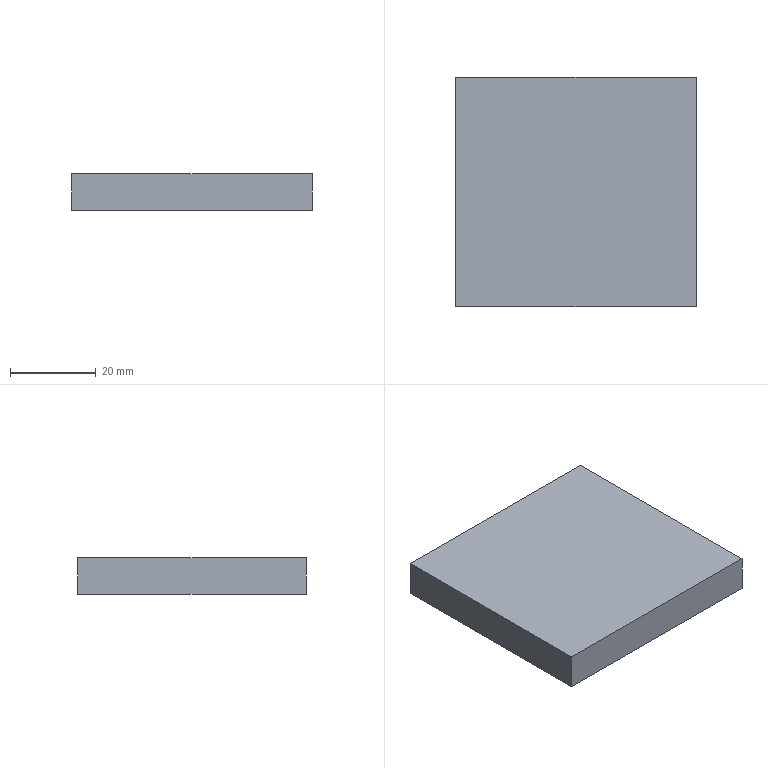NC program | NX | posted with a generic post | part box 56 x 53.3 x 8.5 mm
Lines 1 to 589 of 2943:
N10 G17 G21 G94 G90
(CAVITY_MILL_COPY_1 , TOOL : D6)
N12 T12 M6
N14 G54
N16 G17 G0 G90 X3.464 Y-2.284 S9500 M3
N18 G43 Z30. H12
N20 Z1.
N22 G94 G1 X3.837 Y-1.928 Z0.973 F800.
N24 X5.899 Y-0.453 Z0.84
N26 X6.766 Y0. Z0.789
N28 X5.899 Y0.453 Z0.738
N30 X3.837 Y1.928 Z0.605
N32 X2.861 Y2.861 Z0.534
N34 X1.928 Y3.837 Z0.463
N36 X0.453 Y5.899 Z0.33
N38 X0. Y6.766 Z0.279
N40 X-0.453 Y5.899 Z0.228
N42 X-1.928 Y3.837 Z0.095
N44 X-2.861 Y2.861 Z0.024
N46 X-3.837 Y1.928 Z-0.047
N48 X-5.899 Y0.453 Z-0.18
N50 X-6.766 Y0. Z-0.231
N52 X-5.899 Y-0.453 Z-0.282
N54 X-3.837 Y-1.928 Z-0.415
N56 X-2.995 Y-2.732 Z-0.476
N58 X-2.864 Y-2.864 Z-0.486
N60 X-0.318 Y-0.318
N62 G2 X0. Y-0.644 R19.55 F2500.
N64 X0.644 Y0. R19.55
N66 X0. Y0.644 R19.55
N68 X-0.644 Y0. R19.55
N70 X-0.318 Y-0.318 R19.55
N72 G1 X-2.864 Y-2.864
N74 G2 X0. Y-6.766 R15.95
N76 X6.766 Y0. R15.95
N78 X0. Y6.766 R15.95
N80 X-6.766 Y0. R15.95
N82 X-2.864 Y-2.864 R15.95
N84 G1 X-5.409 Y-5.409
N86 G2 X-2.162 Y-11.142 R12.35
N88 G3 X2.162 Y-11.142 R11.35
N90 G2 X11.73 Y-2.03 R12.35
N92 X12.671 Y-0.857 R11.3
N94 G3 X12.671 Y0.857 R12.7
N96 G2 X11.73 Y2.03 R11.3
N98 X2.162 Y11.142 R12.35
N100 G3 X-2.162 Y11.142 R11.35
N102 G2 X-11.73 Y2.03 R12.35
N104 X-12.671 Y0.857 R11.3
N106 G3 X-12.671 Y-0.857 R12.7
N108 G2 X-11.73 Y-2.03 R11.3
N110 X-5.409 Y-5.409 R12.35
N112 G1 X-7.955 Y-7.955
N114 G2 X-5.394 Y-13.943 R8.75
N116 G3 X5.394 Y-13.943 R14.95
N118 G2 X13.949 Y-5.394 R8.75
N120 X16.098 Y-2.557 R7.7
N122 G3 X16.098 Y2.557 R16.3
N124 G2 X13.949 Y5.394 R7.7
N126 X5.394 Y13.943 R8.75
N128 G3 X-5.394 Y13.943 R14.95
N130 G2 X-13.949 Y5.394 R8.75
N132 X-16.098 Y2.557 R7.7
N134 G3 X-16.098 Y-2.557 R16.3
N136 G2 X-13.949 Y-5.394 R7.7
N138 X-7.955 Y-7.955 R8.75
N140 G1 X-10.501 Y-10.501
N142 G2 X-9.348 Y-16.023 R5.15
N144 G3 X9.348 Y-16.022 R18.55
N146 G2 X16.023 Y-9.348 R5.15
N148 G3 X17.194 Y-6.961 R18.55
N150 G2 X19.323 Y-4.756 R4.1
N152 G3 X19.323 Y4.756 R19.9
N154 G2 X17.194 Y6.961 R4.1
N156 G3 X16.022 Y9.348 R18.55
N158 G2 X9.348 Y16.023 R5.15
N160 G3 X-9.348 Y16.023 R18.55
N162 G2 X-16.023 Y9.348 R5.15
N164 G3 X-17.194 Y6.961 R18.55
N166 G2 X-19.297 Y4.768 R4.1
N168 G1 X-19.325 Y4.75
N170 G3 X-19.325 Y-4.75 R19.9
N172 G1 X-19.297 Y-4.768
N174 G2 X-17.194 Y-6.961 R4.1
N176 G3 X-16.023 Y-9.348 R18.55
N178 G2 X-10.501 Y-10.501 R5.15
N180 G3 X-9.535 Y-10.759 R1.
N182 G1 Z2.514
N184 X-2.284 Y-3.464 Z0.514 F6000.
N186 X-1.928 Y-3.837 Z0.487 F800.
N188 X-0.453 Y-5.899 Z0.354
N190 X0. Y-6.766 Z0.303
N192 X0.453 Y-5.899 Z0.252
N194 X1.928 Y-3.837 Z0.119
N196 X2.861 Y-2.861 Z0.048
N198 X3.837 Y-1.928 Z-0.023
N200 X5.899 Y-0.453 Z-0.155
N202 X6.766 Y0. Z-0.207
N204 X5.899 Y0.453 Z-0.258
N206 X3.837 Y1.928 Z-0.391
N208 X2.861 Y2.861 Z-0.462
N210 X1.928 Y3.837 Z-0.532
N212 X0.453 Y5.899 Z-0.665
N214 X0. Y6.766 Z-0.717
N216 X-0.453 Y5.899 Z-0.768
N218 X-1.928 Y3.837 Z-0.901
N220 X-2.732 Y2.995 Z-0.962
N222 X-2.864 Y2.864 Z-0.971
N224 X-0.318 Y0.318
N226 G2 X-0.644 Y0. R19.55 F2500.
N228 X0. Y-0.644 R19.55
N230 X0.644 Y0. R19.55
N232 X0. Y0.644 R19.55
N234 X-0.318 Y0.318 R19.55
N236 G1 X-2.864 Y2.864
N238 G2 X-6.766 Y0. R15.95
N240 X0. Y-6.766 R15.95
N242 X6.766 Y0. R15.95
N244 X0. Y6.766 R15.95
N246 X-2.864 Y2.864 R15.95
N248 G1 X-5.409 Y5.409
N250 G2 X-11.73 Y2.03 R12.35
N252 X-12.671 Y0.857 R11.3
N254 G3 X-12.671 Y-0.857 R12.7
N256 G2 X-11.73 Y-2.03 R11.3
N258 X-2.162 Y-11.142 R12.35
N260 G3 X2.162 Y-11.142 R11.35
N262 G2 X11.73 Y-2.03 R12.35
N264 X12.671 Y-0.857 R11.3
N266 G3 X12.671 Y0.857 R12.7
N268 G2 X11.73 Y2.03 R11.3
N270 X2.162 Y11.142 R12.35
N272 G3 X-2.162 Y11.142 R11.35
N274 G2 X-5.409 Y5.409 R12.35
N276 G1 X-7.955 Y7.955
N278 G2 X-13.949 Y5.394 R8.75
N280 X-16.098 Y2.557 R7.7
N282 G3 X-16.098 Y-2.557 R16.3
N284 G2 X-13.949 Y-5.394 R7.7
N286 X-5.394 Y-13.943 R8.75
N288 G3 X5.394 Y-13.943 R14.95
N290 G2 X13.949 Y-5.394 R8.75
N292 X16.098 Y-2.557 R7.7
N294 G3 X16.098 Y2.557 R16.3
N296 G2 X13.949 Y5.394 R7.7
N298 X5.394 Y13.943 R8.75
N300 G3 X-5.394 Y13.943 R14.95
N302 G2 X-7.955 Y7.955 R8.75
N304 G1 X-10.501 Y10.501
N306 G2 X-16.023 Y9.348 R5.15
N308 G3 X-17.194 Y6.961 R18.55
N310 G2 X-19.297 Y4.768 R4.1
N312 G1 X-19.325 Y4.75
N314 G3 X-19.325 Y-4.75 R19.9
N316 G1 X-19.297 Y-4.768
N318 G2 X-17.194 Y-6.961 R4.1
N320 G3 X-16.023 Y-9.348 R18.55
N322 G2 X-11.865 Y-9.523 R5.15
N324 X-9.347 Y-16.023 R5.15
N326 G3 X9.348 Y-16.022 R18.55
N328 G2 X16.023 Y-9.348 R5.15
N330 G3 X17.194 Y-6.961 R18.55
N332 G2 X19.323 Y-4.756 R4.1
N334 G3 X19.323 Y4.756 R19.9
N336 G2 X17.194 Y6.961 R4.1
N338 G3 X16.022 Y9.348 R18.55
N340 G2 X9.348 Y16.023 R5.15
N342 G3 X-9.348 Y16.023 R18.55
N344 G2 X-10.501 Y10.501 R5.15
N346 G3 X-10.63 Y10.276 R0.5
N348 G1 Z2.029
N350 X3.464 Y-2.284 Z0.029 F6000.
N352 X3.837 Y-1.928 Z0.002 F800.
N354 X5.899 Y-0.453 Z-0.131
N356 X6.766 Y0. Z-0.183
N358 X5.899 Y0.453 Z-0.234
N360 X3.837 Y1.928 Z-0.367
N362 X2.861 Y2.861 Z-0.438
N364 X1.928 Y3.837 Z-0.508
N366 X0.453 Y5.899 Z-0.641
N368 X0. Y6.766 Z-0.692
N370 X-0.453 Y5.899 Z-0.744
N372 X-1.928 Y3.837 Z-0.877
N374 X-2.861 Y2.861 Z-0.947
N376 X-3.837 Y1.928 Z-1.018
N378 X-5.899 Y0.453 Z-1.151
N380 X-6.766 Y0. Z-1.202
N382 X-5.899 Y-0.453 Z-1.254
N384 X-3.837 Y-1.928 Z-1.386
N386 X-2.995 Y-2.732 Z-1.447
N388 X-2.864 Y-2.864 Z-1.457
N390 X-0.318 Y-0.318
N392 G2 X0. Y-0.644 R19.55 F2500.
N394 X0.644 Y0. R19.55
N396 X0. Y0.644 R19.55
N398 X-0.644 Y0. R19.55
N400 X-0.318 Y-0.318 R19.55
N402 G1 X-2.864 Y-2.864
N404 G2 X0. Y-6.766 R15.95
N406 X6.766 Y0. R15.95
N408 X0. Y6.766 R15.95
N410 X-6.766 Y0. R15.95
N412 X-2.864 Y-2.864 R15.95
N414 G1 X-5.409 Y-5.409
N416 G2 X-2.162 Y-11.142 R12.35
N418 G3 X2.162 Y-11.142 R11.35
N420 G2 X11.73 Y-2.03 R12.35
N422 X12.671 Y-0.857 R11.3
N424 G3 X12.671 Y0.857 R12.7
N426 G2 X11.73 Y2.03 R11.3
N428 X2.162 Y11.142 R12.35
N430 G3 X-2.162 Y11.142 R11.35
N432 G2 X-11.73 Y2.03 R12.35
N434 X-12.671 Y0.857 R11.3
N436 G3 X-12.671 Y-0.857 R12.7
N438 G2 X-11.73 Y-2.03 R11.3
N440 X-5.409 Y-5.409 R12.35
N442 G1 X-7.955 Y-7.955
N444 G2 X-5.394 Y-13.943 R8.75
N446 G3 X5.394 Y-13.943 R14.95
N448 G2 X13.949 Y-5.394 R8.75
N450 X16.098 Y-2.557 R7.7
N452 G3 X16.098 Y2.557 R16.3
N454 G2 X13.949 Y5.394 R7.7
N456 X5.394 Y13.943 R8.75
N458 G3 X-5.394 Y13.943 R14.95
N460 G2 X-13.949 Y5.394 R8.75
N462 X-16.098 Y2.557 R7.7
N464 G3 X-16.098 Y-2.557 R16.3
N466 G2 X-13.949 Y-5.394 R7.7
N468 X-7.955 Y-7.955 R8.75
N470 G1 X-10.501 Y-10.501
N472 G2 X-9.347 Y-16.023 R5.15
N474 G3 X9.348 Y-16.022 R18.55
N476 G2 X16.023 Y-9.348 R5.15
N478 G3 X17.194 Y-6.961 R18.55
N480 G2 X19.323 Y-4.756 R4.1
N482 G3 X19.323 Y4.756 R19.9
N484 G2 X17.194 Y6.961 R4.1
N486 G3 X16.022 Y9.348 R18.55
N488 G2 X9.348 Y16.023 R5.15
N490 G3 X-9.348 Y16.023 R18.55
N492 G2 X-16.023 Y9.348 R5.15
N494 G3 X-17.194 Y6.961 R18.55
N496 G2 X-19.297 Y4.768 R4.1
N498 G1 X-19.325 Y4.75
N500 G3 X-19.325 Y-4.75 R19.9
N502 G1 X-19.297 Y-4.768
N504 G2 X-17.194 Y-6.961 R4.1
N506 G3 X-16.023 Y-9.348 R18.55
N508 G2 X-10.501 Y-10.501 R5.15
N510 G3 X-9.535 Y-10.759 R1.
N512 G1 Z1.543
N514 X-3.464 Y2.284 Z-0.457 F6000.
N516 X-3.837 Y1.928 Z-0.484 F800.
N518 X-5.899 Y0.453 Z-0.617
N520 X-6.766 Y0. Z-0.668
N522 X-5.899 Y-0.453 Z-0.72
N524 X-3.837 Y-1.928 Z-0.852
N526 X-2.861 Y-2.861 Z-0.923
N528 X-1.928 Y-3.837 Z-0.994
N530 X-0.453 Y-5.899 Z-1.127
N532 X0. Y-6.766 Z-1.178
N534 X0.453 Y-5.899 Z-1.229
N536 X1.928 Y-3.837 Z-1.362
N538 X2.861 Y-2.861 Z-1.433
N540 X3.837 Y-1.928 Z-1.504
N542 X5.899 Y-0.453 Z-1.637
N544 X6.766 Y0. Z-1.688
N546 X5.899 Y0.453 Z-1.739
N548 X3.837 Y1.928 Z-1.872
N550 X2.995 Y2.732 Z-1.933
N552 X2.864 Y2.864 Z-1.943
N554 X0.318 Y0.318
N556 G2 X0. Y0.644 R19.55 F2500.
N558 X-0.644 Y0. R19.55
N560 X0. Y-0.644 R19.55
N562 X0.644 Y0. R19.55
N564 X0.318 Y0.318 R19.55
N566 G1 X2.864 Y2.864
N568 G2 X0. Y6.766 R15.95
N570 X-6.766 Y0. R15.95
N572 X0. Y-6.766 R15.95
N574 X6.766 Y0. R15.95
N576 X2.864 Y2.864 R15.95
N578 G1 X5.409 Y5.409
N580 G2 X2.162 Y11.142 R12.35
N582 G3 X-2.162 Y11.142 R11.35
N584 G2 X-11.73 Y2.03 R12.35
N586 X-12.671 Y0.857 R11.3
N588 G3 X-12.671 Y-0.857 R12.7
N590 G2 X-11.73 Y-2.03 R11.3
N592 X-2.162 Y-11.142 R12.35
N594 G3 X2.162 Y-11.142 R11.35
N596 G2 X11.73 Y-2.03 R12.35
N598 X12.671 Y-0.857 R11.3
N600 G3 X12.671 Y0.857 R12.7
N602 G2 X11.73 Y2.03 R11.3
N604 X5.409 Y5.409 R12.35
N606 G1 X7.955 Y7.955
N608 G2 X5.394 Y13.943 R8.75
N610 G3 X-5.394 Y13.943 R14.95
N612 G2 X-13.949 Y5.394 R8.75
N614 X-16.098 Y2.557 R7.7
N616 G3 X-16.098 Y-2.557 R16.3
N618 G2 X-13.949 Y-5.394 R7.7
N620 X-5.394 Y-13.943 R8.75
N622 G3 X5.394 Y-13.943 R14.95
N624 G2 X13.949 Y-5.394 R8.75
N626 X16.098 Y-2.557 R7.7
N628 G3 X16.098 Y2.557 R16.3
N630 G2 X13.949 Y5.394 R7.7
N632 X7.955 Y7.955 R8.75
N634 G1 X10.501 Y10.501
N636 G2 X9.348 Y16.023 R5.15
N638 G3 X-9.348 Y16.023 R18.55
N640 G2 X-16.023 Y9.348 R5.15
N642 G3 X-17.194 Y6.961 R18.55
N644 G2 X-19.297 Y4.768 R4.1
N646 G1 X-19.325 Y4.75
N648 G3 X-19.325 Y-4.75 R19.9
N650 G1 X-19.297 Y-4.768
N652 G2 X-17.194 Y-6.961 R4.1
N654 G3 X-16.023 Y-9.348 R18.55
N656 G2 X-11.865 Y-9.523 R5.15
N658 X-9.347 Y-16.023 R5.151
N660 G3 X9.348 Y-16.022 R18.55
N662 G2 X16.023 Y-9.348 R5.15
N664 G3 X17.194 Y-6.961 R18.55
N666 G2 X19.323 Y-4.756 R4.1
N668 G3 X19.323 Y4.756 R19.9
N670 G2 X17.194 Y6.961 R4.1
N672 G3 X16.022 Y9.348 R18.55
N674 G2 X10.501 Y10.501 R5.15
N676 G3 X9.535 Y10.759 R1.
N678 G1 Z1.057
N680 X3.464 Y-2.284 Z-0.943 F6000.
N682 X3.837 Y-1.928 Z-0.97 F800.
N684 X5.899 Y-0.453 Z-1.103
N686 X6.766 Y0. Z-1.154
N688 X5.899 Y0.453 Z-1.205
N690 X3.837 Y1.928 Z-1.338
N692 X2.861 Y2.861 Z-1.409
N694 X1.928 Y3.837 Z-1.48
N696 X0.453 Y5.899 Z-1.613
N698 X0. Y6.766 Z-1.664
N700 X-0.453 Y5.899 Z-1.715
N702 X-1.928 Y3.837 Z-1.848
N704 X-2.861 Y2.861 Z-1.919
N706 X-3.837 Y1.928 Z-1.99
N708 X-5.899 Y0.453 Z-2.122
N710 X-6.766 Y0. Z-2.174
N712 X-5.899 Y-0.453 Z-2.225
N714 X-3.837 Y-1.928 Z-2.358
N716 X-2.995 Y-2.732 Z-2.419
N718 X-2.864 Y-2.864 Z-2.429
N720 X-0.318 Y-0.318
N722 G2 X0. Y-0.644 R19.55 F2500.
N724 X0.644 Y0. R19.55
N726 X0. Y0.644 R19.55
N728 X-0.644 Y0. R19.55
N730 X-0.318 Y-0.318 R19.55
N732 G1 X-2.864 Y-2.864
N734 G2 X0. Y-6.766 R15.95
N736 X6.766 Y0. R15.95
N738 X0. Y6.766 R15.95
N740 X-6.766 Y0. R15.95
N742 X-2.864 Y-2.864 R15.95
N744 G1 X-5.409 Y-5.409
N746 G2 X-2.162 Y-11.142 R12.35
N748 G3 X2.162 Y-11.142 R11.35
N750 G2 X11.73 Y-2.03 R12.35
N752 X12.671 Y-0.857 R11.3
N754 G3 X12.671 Y0.857 R12.7
N756 G2 X11.73 Y2.03 R11.3
N758 X2.162 Y11.142 R12.35
N760 G3 X-2.162 Y11.142 R11.35
N762 G2 X-11.73 Y2.03 R12.35
N764 X-12.671 Y0.857 R11.3
N766 G3 X-12.671 Y-0.857 R12.7
N768 G2 X-11.73 Y-2.03 R11.3
N770 X-5.409 Y-5.409 R12.35
N772 G1 X-7.955 Y-7.955
N774 G2 X-5.394 Y-13.943 R8.75
N776 G3 X5.394 Y-13.943 R14.95
N778 G2 X13.949 Y-5.394 R8.75
N780 X16.098 Y-2.557 R7.7
N782 G3 X16.098 Y2.557 R16.3
N784 G2 X13.949 Y5.394 R7.7
N786 X5.394 Y13.943 R8.75
N788 G3 X-5.394 Y13.943 R14.95
N790 G2 X-13.949 Y5.394 R8.75
N792 X-16.098 Y2.557 R7.7
N794 G3 X-16.098 Y-2.557 R16.3
N796 G2 X-13.949 Y-5.394 R7.7
N798 X-7.955 Y-7.955 R8.75
N800 G1 X-10.501 Y-10.501
N802 G2 X-9.347 Y-16.023 R5.151
N804 G3 X9.347 Y-16.022 R18.55
N806 G2 X16.023 Y-9.348 R5.15
N808 G3 X17.194 Y-6.961 R18.55
N810 G2 X19.323 Y-4.756 R4.1
N812 G3 X19.323 Y4.756 R19.9
N814 G2 X17.194 Y6.961 R4.1
N816 G3 X16.022 Y9.347 R18.55
N818 G2 X9.348 Y16.023 R5.15
N820 G3 X-9.348 Y16.023 R18.55
N822 G2 X-16.023 Y9.348 R5.15
N824 G3 X-17.194 Y6.961 R18.55
N826 G2 X-19.297 Y4.768 R4.1
N828 G1 X-19.325 Y4.75
N830 G3 X-19.325 Y-4.75 R19.9
N832 G1 X-19.297 Y-4.768
N834 G2 X-17.194 Y-6.961 R4.1
N836 G3 X-16.023 Y-9.348 R18.55
N838 G2 X-10.501 Y-10.501 R5.15
N840 G3 X-9.535 Y-10.759 R1.
N842 G1 Z0.571
N844 X3.464 Y-2.284 Z-1.429 F6000.
N846 X3.837 Y-1.928 Z-1.456 F800.
N848 X5.899 Y-0.453 Z-1.588
N850 X6.766 Y0. Z-1.64
N852 X5.899 Y0.453 Z-1.691
N854 X3.837 Y1.928 Z-1.824
N856 X2.861 Y2.861 Z-1.895
N858 X1.928 Y3.837 Z-1.965
N860 X0.453 Y5.899 Z-2.098
N862 X0. Y6.766 Z-2.15
N864 X-0.453 Y5.899 Z-2.201
N866 X-1.928 Y3.837 Z-2.334
N868 X-2.861 Y2.861 Z-2.404
N870 X-3.837 Y1.928 Z-2.475
N872 X-5.899 Y0.453 Z-2.608
N874 X-6.766 Y0. Z-2.659
N876 X-5.899 Y-0.453 Z-2.711
N878 X-3.837 Y-1.928 Z-2.844
N880 X-2.995 Y-2.732 Z-2.905
N882 X-2.864 Y-2.864 Z-2.914
N884 X-0.318 Y-0.318
N886 G2 X0. Y-0.644 R19.55 F2500.
N888 X0.644 Y0. R19.55
N890 X0. Y0.644 R19.55
N892 X-0.644 Y0. R19.55
N894 X-0.318 Y-0.318 R19.55
N896 G1 X-2.864 Y-2.864
N898 G2 X0. Y-6.766 R15.95
N900 X6.766 Y0. R15.95
N902 X0. Y6.766 R15.95
N904 X-6.766 Y0. R15.95
N906 X-2.864 Y-2.864 R15.95
N908 G1 X-5.409 Y-5.409
N910 G2 X-2.162 Y-11.142 R12.35
N912 G3 X2.162 Y-11.142 R11.35
N914 G2 X11.73 Y-2.03 R12.35
N916 X12.671 Y-0.857 R11.3
N918 G3 X12.671 Y0.857 R12.7
N920 G2 X11.73 Y2.03 R11.3
N922 X2.162 Y11.142 R12.35
N924 G3 X-2.162 Y11.142 R11.35
N926 G2 X-11.73 Y2.03 R12.35
N928 X-12.671 Y0.857 R11.3
N930 G3 X-12.671 Y-0.857 R12.7
N932 G2 X-11.73 Y-2.03 R11.3
N934 X-5.409 Y-5.409 R12.35
N936 G1 X-7.955 Y-7.955
N938 G2 X-5.394 Y-13.943 R8.75
N940 G3 X5.394 Y-13.943 R14.95
N942 G2 X13.949 Y-5.394 R8.75
N944 X16.098 Y-2.557 R7.7
N946 G3 X16.098 Y2.557 R16.3
N948 G2 X13.949 Y5.394 R7.7
N950 X5.394 Y13.943 R8.75
N952 G3 X-5.394 Y13.943 R14.95
N954 G2 X-13.949 Y5.394 R8.75
N956 X-16.098 Y2.557 R7.7
N958 G3 X-16.098 Y-2.557 R16.3
N960 G2 X-13.949 Y-5.394 R7.7
N962 X-7.955 Y-7.955 R8.75
N964 G1 X-10.501 Y-10.501
N966 G2 X-9.347 Y-16.023 R5.151
N968 G3 X9.347 Y-16.022 R18.55
N970 G2 X16.023 Y-9.348 R5.15
N972 G3 X17.194 Y-6.961 R18.55
N974 G2 X19.323 Y-4.756 R4.1
N976 G3 X19.323 Y4.756 R19.9
N978 G2 X17.194 Y6.961 R4.1
N980 G3 X16.022 Y9.347 R18.55
N982 G2 X9.348 Y16.023 R5.15
N984 G3 X-9.348 Y16.023 R18.55
N986 G2 X-16.023 Y9.348 R5.15
N988 G3 X-17.194 Y6.961 R18.55
N990 G2 X-19.311 Y4.762 R4.1
N992 G1 X-19.325 Y4.75
N994 G3 X-19.325 Y-4.75 R19.9
N996 G1 X-19.311 Y-4.762
N998 G2 X-17.194 Y-6.961 R4.1
N1000 G3 X-16.023 Y-9.348 R18.55
N1002 G2 X-10.501 Y-10.501 R5.15
N1004 G3 X-9.535 Y-10.759 R1.
N1006 G1 Z0.086
N1008 X-3.464 Y2.284 Z-1.914 F6000.
N1010 X-3.837 Y1.928 Z-1.941 F800.
N1012 X-5.899 Y0.453 Z-2.074
N1014 X-6.766 Y0. Z-2.125
N1016 X-5.899 Y-0.453 Z-2.177
N1018 X-3.837 Y-1.928 Z-2.31
N1020 X-2.861 Y-2.861 Z-2.38
N1022 X-1.928 Y-3.837 Z-2.451
N1024 X-0.453 Y-5.899 Z-2.584
N1026 X0. Y-6.766 Z-2.635
N1028 X0.453 Y-5.899 Z-2.687
N1030 X1.928 Y-3.837 Z-2.819
N1032 X2.861 Y-2.861 Z-2.89
N1034 X3.837 Y-1.928 Z-2.961
N1036 X5.899 Y-0.453 Z-3.094
N1038 X6.766 Y0. Z-3.145
N1040 X5.899 Y0.453 Z-3.196
N1042 X3.837 Y1.928 Z-3.329
N1044 X2.995 Y2.732 Z-3.39
N1046 X2.864 Y2.864 Z-3.4
N1048 X0.318 Y0.318
N1050 G2 X0. Y0.644 R19.55 F2500.
N1052 X-0.644 Y0. R19.55
N1054 X0. Y-0.644 R19.55
N1056 X0.644 Y0. R19.55
N1058 X0.318 Y0.318 R19.55
N1060 G1 X2.864 Y2.864
N1062 G2 X0. Y6.766 R15.95
N1064 X-6.766 Y0. R15.95
N1066 X0. Y-6.766 R15.95
N1068 X6.766 Y0. R15.95
N1070 X2.864 Y2.864 R15.95
N1072 G1 X5.409 Y5.409
N1074 G2 X2.162 Y11.142 R12.35
N1076 G3 X-2.162 Y11.142 R11.35
N1078 G2 X-11.73 Y2.03 R12.35
N1080 X-12.671 Y0.857 R11.3
N1082 G3 X-12.671 Y-0.857 R12.7
N1084 G2 X-11.73 Y-2.03 R11.3
N1086 X-2.162 Y-11.142 R12.35
N1088 G3 X2.162 Y-11.142 R11.35
N1090 G2 X11.73 Y-2.03 R12.35
N1092 X12.671 Y-0.857 R11.3
N1094 G3 X12.671 Y0.857 R12.7
N1096 G2 X11.73 Y2.03 R11.3
N1098 X5.409 Y5.409 R12.35
N1100 G1 X7.955 Y7.955
N1102 G2 X5.394 Y13.943 R8.75
N1104 G3 X-5.394 Y13.943 R14.95
N1106 G2 X-13.949 Y5.394 R8.75
N1108 X-16.098 Y2.557 R7.7
N1110 G3 X-16.098 Y-2.557 R16.3
N1112 G2 X-13.949 Y-5.394 R7.7
N1114 X-5.394 Y-13.943 R8.75
N1116 G3 X5.394 Y-13.943 R14.95
N1118 G2 X13.949 Y-5.394 R8.75
N1120 X16.098 Y-2.557 R7.7
N1122 G3 X16.098 Y2.557 R16.3
N1124 G2 X13.949 Y5.394 R7.7
N1126 X7.955 Y7.955 R8.75
N1128 G1 X10.501 Y10.501
N1130 G2 X9.348 Y16.023 R5.15
N1132 G3 X-9.348 Y16.023 R18.55
N1134 G2 X-16.023 Y9.348 R5.15
N1136 G3 X-17.194 Y6.961 R18.55
N1138 G2 X-19.31 Y4.762 R4.1
N1140 G1 X-19.325 Y4.75
N1142 G3 X-19.325 Y-4.75 R19.9
N1144 G1 X-19.31 Y-4.762
N1146 G2 X-17.194 Y-6.961 R4.1
N1148 G3 X-16.023 Y-9.348 R18.55
N1150 G2 X-11.865 Y-9.523 R5.15
N1152 X-9.347 Y-16.023 R5.151
N1154 G3 X9.347 Y-16.022 R18.55
N1156 G2 X16.023 Y-9.348 R5.15
N1158 G3 X17.194 Y-6.961 R18.55
N1160 G2 X19.323 Y-4.756 R4.1
N1162 G3 X19.323 Y4.756 R19.9
N1164 G2 X17.194 Y6.961 R4.1
N1166 G3 X16.022 Y9.347 R18.55
N1168 G2 X10.501 Y10.501 R5.15
N1170 G3 X9.535 Y10.759 R1.
N1172 G1 Z-0.4
N1174 G0 Z30.
N1176 M5